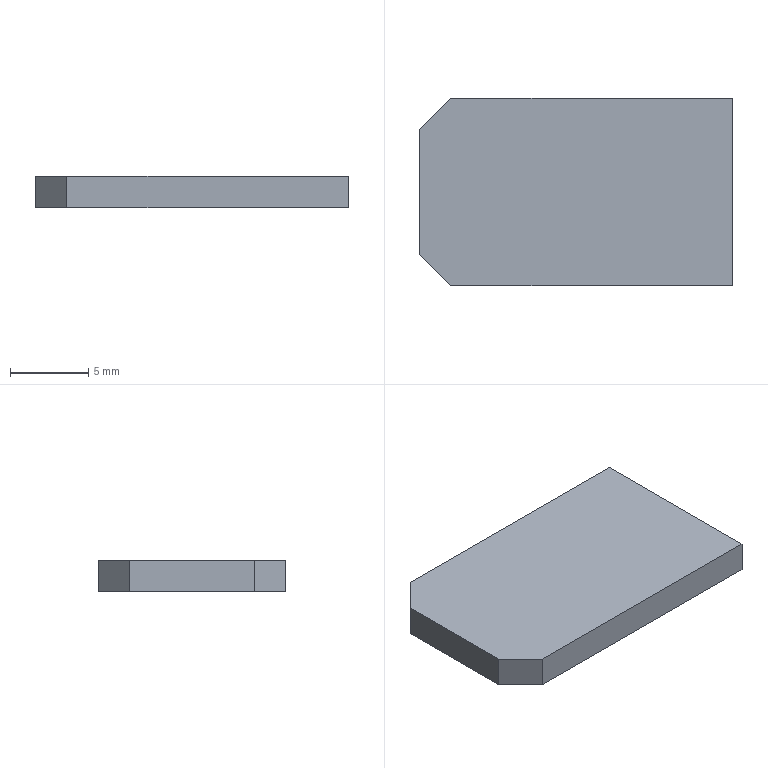Part | STEP file | ASND-0110-Body 1-14 | 1 solid | 8 faces | box 20 x 12 x 2 mm | volume 472 mm3 | plane 8
STEP:
#1=CARTESIAN_POINT('',(0.,0.,0.));
#2=DIRECTION('',(0.,0.,1.));
#3=DIRECTION('',(1.,0.,0.));
#4=AXIS2_PLACEMENT_3D('',#1,#2,#3);
#5=CARTESIAN_POINT('',(0.,10.,2.));
#6=VERTEX_POINT('',#5);
#7=CARTESIAN_POINT('',(2.,12.,2.));
#8=VERTEX_POINT('',#7);
#9=CARTESIAN_POINT('',(2.,12.,2.));
#10=DIRECTION('',(0.7071,0.7071,0.));
#11=VECTOR('',#10,1.);
#12=LINE('',#9,#11);
#13=CARTESIAN_POINT('',(1.,11.,0.));
#14=DIRECTION('',(-0.7071,0.7071,0.));
#15=DIRECTION('',(0.5774,0.5774,0.5774));
#16=AXIS2_PLACEMENT_3D('',#13,#14,#15);
#17=PLANE('',#16);
#18=CARTESIAN_POINT('',(2.309,-0.8165));
#19=DIRECTION('',(0.8165,0.5774));
#20=VECTOR('',#19,1.);
#21=LINE('',#18,#20);
#22=(GEOMETRIC_REPRESENTATION_CONTEXT(2)PARAMETRIC_REPRESENTATION_CONTEXT()REPRESENTATION_CONTEXT('',''));
#23=DEFINITIONAL_REPRESENTATION('',(#21),#22);
#24=PCURVE('',#17,#23);
#25=CARTESIAN_POINT('',(10.,6.,2.));
#26=DIRECTION('',(0.,0.,1.));
#27=DIRECTION('',(0.7071,0.7071,0.));
#28=AXIS2_PLACEMENT_3D('',#25,#26,#27);
#29=PLANE('',#28);
#30=CARTESIAN_POINT('',(-1.414,9.899));
#31=DIRECTION('',(1.,0.));
#32=VECTOR('',#31,1.);
#33=LINE('',#30,#32);
#34=(GEOMETRIC_REPRESENTATION_CONTEXT(2)PARAMETRIC_REPRESENTATION_CONTEXT()REPRESENTATION_CONTEXT('',''));
#35=DEFINITIONAL_REPRESENTATION('',(#33),#34);
#36=PCURVE('',#29,#35);
#37=SURFACE_CURVE('',#12,(#24,#36),.PCURVE_S1.);
#38=EDGE_CURVE('',#6,#8,#37,.T.);
#39=ORIENTED_EDGE('',*,*,#38,.T.);
#40=CARTESIAN_POINT('',(2.,12.,0.));
#41=VERTEX_POINT('',#40);
#42=CARTESIAN_POINT('',(2.,12.,0.));
#43=DIRECTION('',(0.,0.,-1.));
#44=VECTOR('',#43,1.);
#45=LINE('',#42,#44);
#46=CARTESIAN_POINT('',(1.155,0.8165));
#47=DIRECTION('',(-0.5774,0.8165));
#48=VECTOR('',#47,1.);
#49=LINE('',#46,#48);
#50=(GEOMETRIC_REPRESENTATION_CONTEXT(2)PARAMETRIC_REPRESENTATION_CONTEXT()REPRESENTATION_CONTEXT('',''));
#51=DEFINITIONAL_REPRESENTATION('',(#49),#50);
#52=PCURVE('',#17,#51);
#53=CARTESIAN_POINT('',(0.,12.,0.));
#54=DIRECTION('',(0.,1.,0.));
#55=DIRECTION('',(0.7071,0.,0.7071));
#56=AXIS2_PLACEMENT_3D('',#53,#54,#55);
#57=PLANE('',#56);
#58=CARTESIAN_POINT('',(1.414,1.414));
#59=DIRECTION('',(-0.7071,0.7071));
#60=VECTOR('',#59,1.);
#61=LINE('',#58,#60);
#62=(GEOMETRIC_REPRESENTATION_CONTEXT(2)PARAMETRIC_REPRESENTATION_CONTEXT()REPRESENTATION_CONTEXT('',''));
#63=DEFINITIONAL_REPRESENTATION('',(#61),#62);
#64=PCURVE('',#57,#63);
#65=SURFACE_CURVE('',#45,(#52,#64),.PCURVE_S1.);
#66=EDGE_CURVE('',#8,#41,#65,.T.);
#67=ORIENTED_EDGE('',*,*,#66,.T.);
#68=CARTESIAN_POINT('',(0.,10.,0.));
#69=VERTEX_POINT('',#68);
#70=CARTESIAN_POINT('',(2.,12.,0.));
#71=DIRECTION('',(-0.7071,-0.7071,0.));
#72=VECTOR('',#71,1.);
#73=LINE('',#70,#72);
#74=CARTESIAN_POINT('',(1.155,0.8165));
#75=DIRECTION('',(-0.8165,-0.5774));
#76=VECTOR('',#75,1.);
#77=LINE('',#74,#76);
#78=(GEOMETRIC_REPRESENTATION_CONTEXT(2)PARAMETRIC_REPRESENTATION_CONTEXT()REPRESENTATION_CONTEXT('',''));
#79=DEFINITIONAL_REPRESENTATION('',(#77),#78);
#80=PCURVE('',#17,#79);
#81=CARTESIAN_POINT('',(10.,6.,0.));
#82=DIRECTION('',(0.,0.,1.));
#83=DIRECTION('',(0.7071,0.7071,0.));
#84=AXIS2_PLACEMENT_3D('',#81,#82,#83);
#85=PLANE('',#84);
#86=CARTESIAN_POINT('',(-1.414,9.899));
#87=DIRECTION('',(-1.,0.));
#88=VECTOR('',#87,1.);
#89=LINE('',#86,#88);
#90=(GEOMETRIC_REPRESENTATION_CONTEXT(2)PARAMETRIC_REPRESENTATION_CONTEXT()REPRESENTATION_CONTEXT('',''));
#91=DEFINITIONAL_REPRESENTATION('',(#89),#90);
#92=PCURVE('',#85,#91);
#93=SURFACE_CURVE('',#73,(#80,#92),.PCURVE_S1.);
#94=EDGE_CURVE('',#41,#69,#93,.T.);
#95=ORIENTED_EDGE('',*,*,#94,.T.);
#96=CARTESIAN_POINT('',(0.,10.,0.));
#97=DIRECTION('',(0.,0.,1.));
#98=VECTOR('',#97,1.);
#99=LINE('',#96,#98);
#100=CARTESIAN_POINT('',(-1.155,-0.8165));
#101=DIRECTION('',(0.5774,-0.8165));
#102=VECTOR('',#101,1.);
#103=LINE('',#100,#102);
#104=(GEOMETRIC_REPRESENTATION_CONTEXT(2)PARAMETRIC_REPRESENTATION_CONTEXT()REPRESENTATION_CONTEXT('',''));
#105=DEFINITIONAL_REPRESENTATION('',(#103),#104);
#106=PCURVE('',#17,#105);
#107=CARTESIAN_POINT('',(0.,0.,0.));
#108=DIRECTION('',(-1.,0.,0.));
#109=DIRECTION('',(0.,0.7071,0.7071));
#110=AXIS2_PLACEMENT_3D('',#107,#108,#109);
#111=PLANE('',#110);
#112=CARTESIAN_POINT('',(7.071,7.071));
#113=DIRECTION('',(0.7071,-0.7071));
#114=VECTOR('',#113,1.);
#115=LINE('',#112,#114);
#116=(GEOMETRIC_REPRESENTATION_CONTEXT(2)PARAMETRIC_REPRESENTATION_CONTEXT()REPRESENTATION_CONTEXT('',''));
#117=DEFINITIONAL_REPRESENTATION('',(#115),#116);
#118=PCURVE('',#111,#117);
#119=SURFACE_CURVE('',#99,(#106,#118),.PCURVE_S1.);
#120=EDGE_CURVE('',#69,#6,#119,.T.);
#121=ORIENTED_EDGE('',*,*,#120,.T.);
#122=EDGE_LOOP('',(#39,#67,#95,#121));
#123=FACE_BOUND('',#122,.T.);
#124=ADVANCED_FACE('',(#123),#17,.T.);
#125=ORIENTED_EDGE('',*,*,#66,.F.);
#126=CARTESIAN_POINT('',(20.,12.,2.));
#127=VERTEX_POINT('',#126);
#128=CARTESIAN_POINT('',(20.,12.,2.));
#129=DIRECTION('',(1.,0.,0.));
#130=VECTOR('',#129,1.);
#131=LINE('',#128,#130);
#132=CARTESIAN_POINT('',(15.556,12.728));
#133=DIRECTION('',(0.7071,0.7071));
#134=VECTOR('',#133,1.);
#135=LINE('',#132,#134);
#136=(GEOMETRIC_REPRESENTATION_CONTEXT(2)PARAMETRIC_REPRESENTATION_CONTEXT()REPRESENTATION_CONTEXT('',''));
#137=DEFINITIONAL_REPRESENTATION('',(#135),#136);
#138=PCURVE('',#57,#137);
#139=CARTESIAN_POINT('',(11.314,-2.828));
#140=DIRECTION('',(0.7071,-0.7071));
#141=VECTOR('',#140,1.);
#142=LINE('',#139,#141);
#143=(GEOMETRIC_REPRESENTATION_CONTEXT(2)PARAMETRIC_REPRESENTATION_CONTEXT()REPRESENTATION_CONTEXT('',''));
#144=DEFINITIONAL_REPRESENTATION('',(#142),#143);
#145=PCURVE('',#29,#144);
#146=SURFACE_CURVE('',#131,(#138,#145),.PCURVE_S1.);
#147=EDGE_CURVE('',#8,#127,#146,.T.);
#148=ORIENTED_EDGE('',*,*,#147,.T.);
#149=CARTESIAN_POINT('',(20.,12.,0.));
#150=VERTEX_POINT('',#149);
#151=CARTESIAN_POINT('',(20.,12.,0.));
#152=DIRECTION('',(0.,0.,1.));
#153=VECTOR('',#152,1.);
#154=LINE('',#151,#153);
#155=CARTESIAN_POINT('',(14.142,14.142));
#156=DIRECTION('',(0.7071,-0.7071));
#157=VECTOR('',#156,1.);
#158=LINE('',#155,#157);
#159=(GEOMETRIC_REPRESENTATION_CONTEXT(2)PARAMETRIC_REPRESENTATION_CONTEXT()REPRESENTATION_CONTEXT('',''));
#160=DEFINITIONAL_REPRESENTATION('',(#158),#159);
#161=PCURVE('',#57,#160);
#162=CARTESIAN_POINT('',(20.,12.,0.));
#163=DIRECTION('',(1.,0.,0.));
#164=DIRECTION('',(0.,0.7071,0.7071));
#165=AXIS2_PLACEMENT_3D('',#162,#163,#164);
#166=PLANE('',#165);
#167=CARTESIAN_POINT('',(0.,0.));
#168=DIRECTION('',(0.7071,0.7071));
#169=VECTOR('',#168,1.);
#170=LINE('',#167,#169);
#171=(GEOMETRIC_REPRESENTATION_CONTEXT(2)PARAMETRIC_REPRESENTATION_CONTEXT()REPRESENTATION_CONTEXT('',''));
#172=DEFINITIONAL_REPRESENTATION('',(#170),#171);
#173=PCURVE('',#166,#172);
#174=SURFACE_CURVE('',#154,(#161,#173),.PCURVE_S1.);
#175=EDGE_CURVE('',#150,#127,#174,.T.);
#176=ORIENTED_EDGE('',*,*,#175,.F.);
#177=CARTESIAN_POINT('',(20.,12.,0.));
#178=DIRECTION('',(-1.,0.,0.));
#179=VECTOR('',#178,1.);
#180=LINE('',#177,#179);
#181=CARTESIAN_POINT('',(14.142,14.142));
#182=DIRECTION('',(-0.7071,-0.7071));
#183=VECTOR('',#182,1.);
#184=LINE('',#181,#183);
#185=(GEOMETRIC_REPRESENTATION_CONTEXT(2)PARAMETRIC_REPRESENTATION_CONTEXT()REPRESENTATION_CONTEXT('',''));
#186=DEFINITIONAL_REPRESENTATION('',(#184),#185);
#187=PCURVE('',#57,#186);
#188=CARTESIAN_POINT('',(11.314,-2.828));
#189=DIRECTION('',(-0.7071,0.7071));
#190=VECTOR('',#189,1.);
#191=LINE('',#188,#190);
#192=(GEOMETRIC_REPRESENTATION_CONTEXT(2)PARAMETRIC_REPRESENTATION_CONTEXT()REPRESENTATION_CONTEXT('',''));
#193=DEFINITIONAL_REPRESENTATION('',(#191),#192);
#194=PCURVE('',#85,#193);
#195=SURFACE_CURVE('',#180,(#187,#194),.PCURVE_S1.);
#196=EDGE_CURVE('',#150,#41,#195,.T.);
#197=ORIENTED_EDGE('',*,*,#196,.T.);
#198=EDGE_LOOP('',(#125,#148,#176,#197));
#199=FACE_BOUND('',#198,.T.);
#200=ADVANCED_FACE('',(#199),#57,.T.);
#201=ORIENTED_EDGE('',*,*,#38,.F.);
#202=CARTESIAN_POINT('',(0.,2.,2.));
#203=VERTEX_POINT('',#202);
#204=CARTESIAN_POINT('',(0.,12.,2.));
#205=DIRECTION('',(0.,1.,0.));
#206=VECTOR('',#205,1.);
#207=LINE('',#204,#206);
#208=CARTESIAN_POINT('',(-2.828,11.314));
#209=DIRECTION('',(0.7071,0.7071));
#210=VECTOR('',#209,1.);
#211=LINE('',#208,#210);
#212=(GEOMETRIC_REPRESENTATION_CONTEXT(2)PARAMETRIC_REPRESENTATION_CONTEXT()REPRESENTATION_CONTEXT('',''));
#213=DEFINITIONAL_REPRESENTATION('',(#211),#212);
#214=PCURVE('',#29,#213);
#215=CARTESIAN_POINT('',(9.899,7.071));
#216=DIRECTION('',(0.7071,0.7071));
#217=VECTOR('',#216,1.);
#218=LINE('',#215,#217);
#219=(GEOMETRIC_REPRESENTATION_CONTEXT(2)PARAMETRIC_REPRESENTATION_CONTEXT()REPRESENTATION_CONTEXT('',''));
#220=DEFINITIONAL_REPRESENTATION('',(#218),#219);
#221=PCURVE('',#111,#220);
#222=SURFACE_CURVE('',#207,(#214,#221),.PCURVE_S1.);
#223=EDGE_CURVE('',#203,#6,#222,.T.);
#224=ORIENTED_EDGE('',*,*,#223,.F.);
#225=CARTESIAN_POINT('',(2.,0.,2.));
#226=VERTEX_POINT('',#225);
#227=CARTESIAN_POINT('',(2.,0.,2.));
#228=DIRECTION('',(-0.7071,0.7071,0.));
#229=VECTOR('',#228,1.);
#230=LINE('',#227,#229);
#231=CARTESIAN_POINT('',(-9.899,1.414));
#232=DIRECTION('',(0.,1.));
#233=VECTOR('',#232,1.);
#234=LINE('',#231,#233);
#235=(GEOMETRIC_REPRESENTATION_CONTEXT(2)PARAMETRIC_REPRESENTATION_CONTEXT()REPRESENTATION_CONTEXT('',''));
#236=DEFINITIONAL_REPRESENTATION('',(#234),#235);
#237=PCURVE('',#29,#236);
#238=CARTESIAN_POINT('',(1.,1.,0.));
#239=DIRECTION('',(-0.7071,-0.7071,0.));
#240=DIRECTION('',(-0.5774,0.5774,0.5774));
#241=AXIS2_PLACEMENT_3D('',#238,#239,#240);
#242=PLANE('',#241);
#243=CARTESIAN_POINT('',(0.,-2.449));
#244=DIRECTION('',(0.8165,0.5774));
#245=VECTOR('',#244,1.);
#246=LINE('',#243,#245);
#247=(GEOMETRIC_REPRESENTATION_CONTEXT(2)PARAMETRIC_REPRESENTATION_CONTEXT()REPRESENTATION_CONTEXT('',''));
#248=DEFINITIONAL_REPRESENTATION('',(#246),#247);
#249=PCURVE('',#242,#248);
#250=SURFACE_CURVE('',#230,(#237,#249),.PCURVE_S1.);
#251=EDGE_CURVE('',#226,#203,#250,.T.);
#252=ORIENTED_EDGE('',*,*,#251,.F.);
#253=CARTESIAN_POINT('',(20.,0.,2.));
#254=VERTEX_POINT('',#253);
#255=CARTESIAN_POINT('',(0.,0.,2.));
#256=DIRECTION('',(-1.,0.,0.));
#257=VECTOR('',#256,1.);
#258=LINE('',#255,#257);
#259=CARTESIAN_POINT('',(-11.314,2.828));
#260=DIRECTION('',(-0.7071,0.7071));
#261=VECTOR('',#260,1.);
#262=LINE('',#259,#261);
#263=(GEOMETRIC_REPRESENTATION_CONTEXT(2)PARAMETRIC_REPRESENTATION_CONTEXT()REPRESENTATION_CONTEXT('',''));
#264=DEFINITIONAL_REPRESENTATION('',(#262),#263);
#265=PCURVE('',#29,#264);
#266=CARTESIAN_POINT('',(20.,0.,0.));
#267=DIRECTION('',(0.,-1.,0.));
#268=DIRECTION('',(0.7071,0.,0.7071));
#269=AXIS2_PLACEMENT_3D('',#266,#267,#268);
#270=PLANE('',#269);
#271=CARTESIAN_POINT('',(-12.728,15.556));
#272=DIRECTION('',(-0.7071,0.7071));
#273=VECTOR('',#272,1.);
#274=LINE('',#271,#273);
#275=(GEOMETRIC_REPRESENTATION_CONTEXT(2)PARAMETRIC_REPRESENTATION_CONTEXT()REPRESENTATION_CONTEXT('',''));
#276=DEFINITIONAL_REPRESENTATION('',(#274),#275);
#277=PCURVE('',#270,#276);
#278=SURFACE_CURVE('',#258,(#265,#277),.PCURVE_S1.);
#279=EDGE_CURVE('',#254,#226,#278,.T.);
#280=ORIENTED_EDGE('',*,*,#279,.F.);
#281=CARTESIAN_POINT('',(20.,0.,2.));
#282=DIRECTION('',(0.,-1.,0.));
#283=VECTOR('',#282,1.);
#284=LINE('',#281,#283);
#285=CARTESIAN_POINT('',(2.828,-11.314));
#286=DIRECTION('',(-0.7071,-0.7071));
#287=VECTOR('',#286,1.);
#288=LINE('',#285,#287);
#289=(GEOMETRIC_REPRESENTATION_CONTEXT(2)PARAMETRIC_REPRESENTATION_CONTEXT()REPRESENTATION_CONTEXT('',''));
#290=DEFINITIONAL_REPRESENTATION('',(#288),#289);
#291=PCURVE('',#29,#290);
#292=CARTESIAN_POINT('',(-7.071,9.899));
#293=DIRECTION('',(-0.7071,0.7071));
#294=VECTOR('',#293,1.);
#295=LINE('',#292,#294);
#296=(GEOMETRIC_REPRESENTATION_CONTEXT(2)PARAMETRIC_REPRESENTATION_CONTEXT()REPRESENTATION_CONTEXT('',''));
#297=DEFINITIONAL_REPRESENTATION('',(#295),#296);
#298=PCURVE('',#166,#297);
#299=SURFACE_CURVE('',#284,(#291,#298),.PCURVE_S1.);
#300=EDGE_CURVE('',#127,#254,#299,.T.);
#301=ORIENTED_EDGE('',*,*,#300,.F.);
#302=ORIENTED_EDGE('',*,*,#147,.F.);
#303=EDGE_LOOP('',(#201,#224,#252,#280,#301,#302));
#304=FACE_BOUND('',#303,.T.);
#305=ADVANCED_FACE('',(#304),#29,.T.);
#306=ORIENTED_EDGE('',*,*,#251,.T.);
#307=CARTESIAN_POINT('',(0.,2.,0.));
#308=VERTEX_POINT('',#307);
#309=CARTESIAN_POINT('',(0.,2.,0.));
#310=DIRECTION('',(0.,0.,-1.));
#311=VECTOR('',#310,1.);
#312=LINE('',#309,#311);
#313=CARTESIAN_POINT('',(1.155,0.8165));
#314=DIRECTION('',(-0.5774,0.8165));
#315=VECTOR('',#314,1.);
#316=LINE('',#313,#315);
#317=(GEOMETRIC_REPRESENTATION_CONTEXT(2)PARAMETRIC_REPRESENTATION_CONTEXT()REPRESENTATION_CONTEXT('',''));
#318=DEFINITIONAL_REPRESENTATION('',(#316),#317);
#319=PCURVE('',#242,#318);
#320=CARTESIAN_POINT('',(1.414,1.414));
#321=DIRECTION('',(-0.7071,0.7071));
#322=VECTOR('',#321,1.);
#323=LINE('',#320,#322);
#324=(GEOMETRIC_REPRESENTATION_CONTEXT(2)PARAMETRIC_REPRESENTATION_CONTEXT()REPRESENTATION_CONTEXT('',''));
#325=DEFINITIONAL_REPRESENTATION('',(#323),#324);
#326=PCURVE('',#111,#325);
#327=SURFACE_CURVE('',#312,(#319,#326),.PCURVE_S1.);
#328=EDGE_CURVE('',#203,#308,#327,.T.);
#329=ORIENTED_EDGE('',*,*,#328,.T.);
#330=CARTESIAN_POINT('',(2.,0.,0.));
#331=VERTEX_POINT('',#330);
#332=CARTESIAN_POINT('',(2.,0.,0.));
#333=DIRECTION('',(0.7071,-0.7071,0.));
#334=VECTOR('',#333,1.);
#335=LINE('',#332,#334);
#336=CARTESIAN_POINT('',(-1.155,-0.8165));
#337=DIRECTION('',(-0.8165,-0.5774));
#338=VECTOR('',#337,1.);
#339=LINE('',#336,#338);
#340=(GEOMETRIC_REPRESENTATION_CONTEXT(2)PARAMETRIC_REPRESENTATION_CONTEXT()REPRESENTATION_CONTEXT('',''));
#341=DEFINITIONAL_REPRESENTATION('',(#339),#340);
#342=PCURVE('',#242,#341);
#343=CARTESIAN_POINT('',(-9.899,1.414));
#344=DIRECTION('',(0.,-1.));
#345=VECTOR('',#344,1.);
#346=LINE('',#343,#345);
#347=(GEOMETRIC_REPRESENTATION_CONTEXT(2)PARAMETRIC_REPRESENTATION_CONTEXT()REPRESENTATION_CONTEXT('',''));
#348=DEFINITIONAL_REPRESENTATION('',(#346),#347);
#349=PCURVE('',#85,#348);
#350=SURFACE_CURVE('',#335,(#342,#349),.PCURVE_S1.);
#351=EDGE_CURVE('',#308,#331,#350,.T.);
#352=ORIENTED_EDGE('',*,*,#351,.T.);
#353=CARTESIAN_POINT('',(2.,0.,0.));
#354=DIRECTION('',(0.,0.,1.));
#355=VECTOR('',#354,1.);
#356=LINE('',#353,#355);
#357=CARTESIAN_POINT('',(-1.155,-0.8165));
#358=DIRECTION('',(0.5774,-0.8165));
#359=VECTOR('',#358,1.);
#360=LINE('',#357,#359);
#361=(GEOMETRIC_REPRESENTATION_CONTEXT(2)PARAMETRIC_REPRESENTATION_CONTEXT()REPRESENTATION_CONTEXT('',''));
#362=DEFINITIONAL_REPRESENTATION('',(#360),#361);
#363=PCURVE('',#242,#362);
#364=CARTESIAN_POINT('',(-12.728,12.728));
#365=DIRECTION('',(0.7071,0.7071));
#366=VECTOR('',#365,1.);
#367=LINE('',#364,#366);
#368=(GEOMETRIC_REPRESENTATION_CONTEXT(2)PARAMETRIC_REPRESENTATION_CONTEXT()REPRESENTATION_CONTEXT('',''));
#369=DEFINITIONAL_REPRESENTATION('',(#367),#368);
#370=PCURVE('',#270,#369);
#371=SURFACE_CURVE('',#356,(#363,#370),.PCURVE_S1.);
#372=EDGE_CURVE('',#331,#226,#371,.T.);
#373=ORIENTED_EDGE('',*,*,#372,.T.);
#374=EDGE_LOOP('',(#306,#329,#352,#373));
#375=FACE_BOUND('',#374,.T.);
#376=ADVANCED_FACE('',(#375),#242,.T.);
#377=ORIENTED_EDGE('',*,*,#372,.F.);
#378=CARTESIAN_POINT('',(20.,0.,0.));
#379=VERTEX_POINT('',#378);
#380=CARTESIAN_POINT('',(0.,0.,0.));
#381=DIRECTION('',(1.,0.,0.));
#382=VECTOR('',#381,1.);
#383=LINE('',#380,#382);
#384=CARTESIAN_POINT('',(-14.142,14.142));
#385=DIRECTION('',(0.7071,-0.7071));
#386=VECTOR('',#385,1.);
#387=LINE('',#384,#386);
#388=(GEOMETRIC_REPRESENTATION_CONTEXT(2)PARAMETRIC_REPRESENTATION_CONTEXT()REPRESENTATION_CONTEXT('',''));
#389=DEFINITIONAL_REPRESENTATION('',(#387),#388);
#390=PCURVE('',#270,#389);
#391=CARTESIAN_POINT('',(-11.314,2.828));
#392=DIRECTION('',(0.7071,-0.7071));
#393=VECTOR('',#392,1.);
#394=LINE('',#391,#393);
#395=(GEOMETRIC_REPRESENTATION_CONTEXT(2)PARAMETRIC_REPRESENTATION_CONTEXT()REPRESENTATION_CONTEXT('',''));
#396=DEFINITIONAL_REPRESENTATION('',(#394),#395);
#397=PCURVE('',#85,#396);
#398=SURFACE_CURVE('',#383,(#390,#397),.PCURVE_S1.);
#399=EDGE_CURVE('',#331,#379,#398,.T.);
#400=ORIENTED_EDGE('',*,*,#399,.T.);
#401=CARTESIAN_POINT('',(20.,0.,0.));
#402=DIRECTION('',(0.,0.,1.));
#403=VECTOR('',#402,1.);
#404=LINE('',#401,#403);
#405=CARTESIAN_POINT('',(0.,0.));
#406=DIRECTION('',(0.7071,0.7071));
#407=VECTOR('',#406,1.);
#408=LINE('',#405,#407);
#409=(GEOMETRIC_REPRESENTATION_CONTEXT(2)PARAMETRIC_REPRESENTATION_CONTEXT()REPRESENTATION_CONTEXT('',''));
#410=DEFINITIONAL_REPRESENTATION('',(#408),#409);
#411=PCURVE('',#270,#410);
#412=CARTESIAN_POINT('',(-8.485,8.485));
#413=DIRECTION('',(0.7071,0.7071));
#414=VECTOR('',#413,1.);
#415=LINE('',#412,#414);
#416=(GEOMETRIC_REPRESENTATION_CONTEXT(2)PARAMETRIC_REPRESENTATION_CONTEXT()REPRESENTATION_CONTEXT('',''));
#417=DEFINITIONAL_REPRESENTATION('',(#415),#416);
#418=PCURVE('',#166,#417);
#419=SURFACE_CURVE('',#404,(#411,#418),.PCURVE_S1.);
#420=EDGE_CURVE('',#379,#254,#419,.T.);
#421=ORIENTED_EDGE('',*,*,#420,.T.);
#422=ORIENTED_EDGE('',*,*,#279,.T.);
#423=EDGE_LOOP('',(#377,#400,#421,#422));
#424=FACE_BOUND('',#423,.T.);
#425=ADVANCED_FACE('',(#424),#270,.T.);
#426=ORIENTED_EDGE('',*,*,#120,.F.);
#427=CARTESIAN_POINT('',(0.,12.,0.));
#428=DIRECTION('',(0.,-1.,0.));
#429=VECTOR('',#428,1.);
#430=LINE('',#427,#429);
#431=CARTESIAN_POINT('',(8.485,8.485));
#432=DIRECTION('',(-0.7071,-0.7071));
#433=VECTOR('',#432,1.);
#434=LINE('',#431,#433);
#435=(GEOMETRIC_REPRESENTATION_CONTEXT(2)PARAMETRIC_REPRESENTATION_CONTEXT()REPRESENTATION_CONTEXT('',''));
#436=DEFINITIONAL_REPRESENTATION('',(#434),#435);
#437=PCURVE('',#111,#436);
#438=CARTESIAN_POINT('',(-2.828,11.314));
#439=DIRECTION('',(-0.7071,-0.7071));
#440=VECTOR('',#439,1.);
#441=LINE('',#438,#440);
#442=(GEOMETRIC_REPRESENTATION_CONTEXT(2)PARAMETRIC_REPRESENTATION_CONTEXT()REPRESENTATION_CONTEXT('',''));
#443=DEFINITIONAL_REPRESENTATION('',(#441),#442);
#444=PCURVE('',#85,#443);
#445=SURFACE_CURVE('',#430,(#437,#444),.PCURVE_S1.);
#446=EDGE_CURVE('',#69,#308,#445,.T.);
#447=ORIENTED_EDGE('',*,*,#446,.T.);
#448=ORIENTED_EDGE('',*,*,#328,.F.);
#449=ORIENTED_EDGE('',*,*,#223,.T.);
#450=EDGE_LOOP('',(#426,#447,#448,#449));
#451=FACE_BOUND('',#450,.T.);
#452=ADVANCED_FACE('',(#451),#111,.T.);
#453=ORIENTED_EDGE('',*,*,#300,.T.);
#454=ORIENTED_EDGE('',*,*,#420,.F.);
#455=CARTESIAN_POINT('',(20.,0.,0.));
#456=DIRECTION('',(0.,1.,0.));
#457=VECTOR('',#456,1.);
#458=LINE('',#455,#457);
#459=CARTESIAN_POINT('',(-8.485,8.485));
#460=DIRECTION('',(0.7071,-0.7071));
#461=VECTOR('',#460,1.);
#462=LINE('',#459,#461);
#463=(GEOMETRIC_REPRESENTATION_CONTEXT(2)PARAMETRIC_REPRESENTATION_CONTEXT()REPRESENTATION_CONTEXT('',''));
#464=DEFINITIONAL_REPRESENTATION('',(#462),#463);
#465=PCURVE('',#166,#464);
#466=CARTESIAN_POINT('',(2.828,-11.314));
#467=DIRECTION('',(0.7071,0.7071));
#468=VECTOR('',#467,1.);
#469=LINE('',#466,#468);
#470=(GEOMETRIC_REPRESENTATION_CONTEXT(2)PARAMETRIC_REPRESENTATION_CONTEXT()REPRESENTATION_CONTEXT('',''));
#471=DEFINITIONAL_REPRESENTATION('',(#469),#470);
#472=PCURVE('',#85,#471);
#473=SURFACE_CURVE('',#458,(#465,#472),.PCURVE_S1.);
#474=EDGE_CURVE('',#379,#150,#473,.T.);
#475=ORIENTED_EDGE('',*,*,#474,.T.);
#476=ORIENTED_EDGE('',*,*,#175,.T.);
#477=EDGE_LOOP('',(#453,#454,#475,#476));
#478=FACE_BOUND('',#477,.T.);
#479=ADVANCED_FACE('',(#478),#166,.T.);
#480=ORIENTED_EDGE('',*,*,#94,.F.);
#481=ORIENTED_EDGE('',*,*,#196,.F.);
#482=ORIENTED_EDGE('',*,*,#474,.F.);
#483=ORIENTED_EDGE('',*,*,#399,.F.);
#484=ORIENTED_EDGE('',*,*,#351,.F.);
#485=ORIENTED_EDGE('',*,*,#446,.F.);
#486=EDGE_LOOP('',(#480,#481,#482,#483,#484,#485));
#487=FACE_BOUND('',#486,.T.);
#488=ADVANCED_FACE('',(#487),#85,.F.);
#489=CLOSED_SHELL('',(#124,#200,#305,#376,#425,#452,#479,#488));
#490=MANIFOLD_SOLID_BREP('',#489);
#491=(LENGTH_UNIT()NAMED_UNIT(*)SI_UNIT(.MILLI.,.METRE.));
#492=UNCERTAINTY_MEASURE_WITH_UNIT(LENGTH_MEASURE(0.0000001),#491,'','');
#493=(NAMED_UNIT(*)PLANE_ANGLE_UNIT()SI_UNIT($,.RADIAN.));
#494=(NAMED_UNIT(*)SI_UNIT($,.STERADIAN.)SOLID_ANGLE_UNIT());
#495=(GEOMETRIC_REPRESENTATION_CONTEXT(3)GLOBAL_UNCERTAINTY_ASSIGNED_CONTEXT((#492))GLOBAL_UNIT_ASSIGNED_CONTEXT((#491,#493,#494))REPRESENTATION_CONTEXT('',''));
#496=ADVANCED_BREP_SHAPE_REPRESENTATION('',(#4,#490),#495);